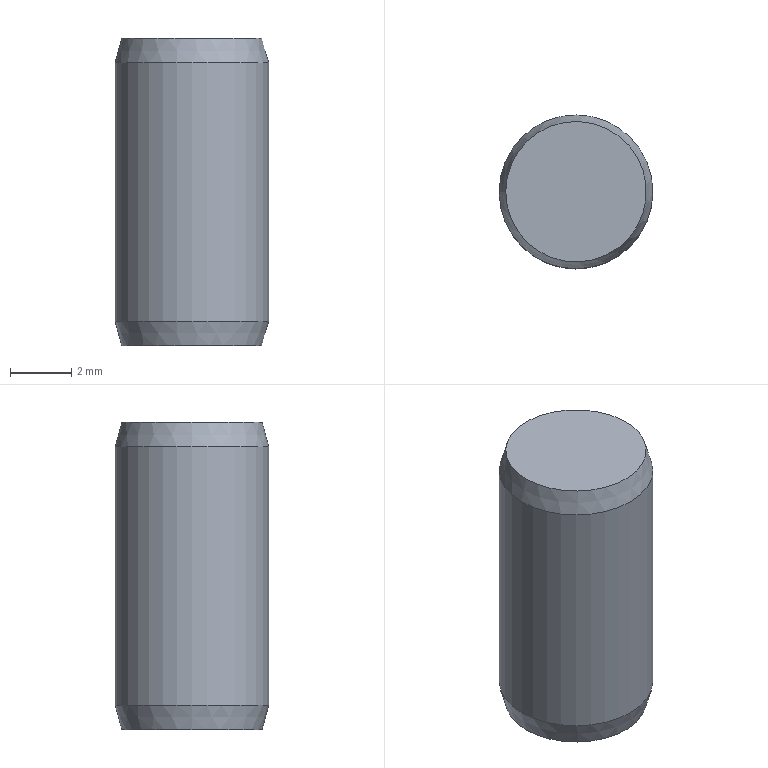Part | NX | features DATUM_CSYS 2, LINE 1, SKETCH 1, SWP104 1 | 1 solid | 5 faces | box 5 x 5 x 10 mm | volume 193.733 mm3 | plane 2 | cone 2 | cylinder 1 | commonest cylinder face diameters 5 x1
STEP:
#1=CARTESIAN_POINT('',(-2.286,0.,-10.));
#2=VERTEX_POINT('',#1);
#3=CARTESIAN_POINT('',(0.,0.,-10.));
#4=DIRECTION('',(0.,0.,-1.));
#5=DIRECTION('',(-1.,0.,0.));
#6=AXIS2_PLACEMENT_3D('',#3,#4,#5);
#7=CIRCLE('',#6,2.286);
#8=EDGE_CURVE('',#2,#2,#7,.T.);
#9=ORIENTED_EDGE('',*,*,#8,.T.);
#10=EDGE_LOOP('',(#9));
#11=FACE_BOUND('',#10,.T.);
#12=CARTESIAN_POINT('',(0.,0.,-10.));
#13=DIRECTION('',(0.,0.,-1.));
#14=DIRECTION('',(-1.,0.,0.));
#15=AXIS2_PLACEMENT_3D('',#12,#13,#14);
#16=PLANE('',#15);
#17=ADVANCED_FACE('',(#11),#16,.T.);
#18=CARTESIAN_POINT('',(-2.5,0.,-9.2));
#19=VERTEX_POINT('',#18);
#20=CARTESIAN_POINT('',(0.,0.,-9.2));
#21=DIRECTION('',(0.,0.,-1.));
#22=DIRECTION('',(-1.,0.,0.));
#23=AXIS2_PLACEMENT_3D('',#20,#21,#22);
#24=CIRCLE('',#23,2.5);
#25=EDGE_CURVE('',#19,#19,#24,.T.);
#26=ORIENTED_EDGE('',*,*,#25,.T.);
#27=EDGE_LOOP('',(#26));
#28=FACE_BOUND('',#27,.T.);
#29=ORIENTED_EDGE('',*,*,#8,.F.);
#30=EDGE_LOOP('',(#29));
#31=FACE_BOUND('',#30,.T.);
#32=CARTESIAN_POINT('',(0.,0.,-10.));
#33=DIRECTION('',(0.,0.,1.));
#34=DIRECTION('',(1.,0.,0.));
#35=AXIS2_PLACEMENT_3D('',#32,#33,#34);
#36=CONICAL_SURFACE('',#35,2.286,0.2618);
#37=ADVANCED_FACE('',(#28,#31),#36,.T.);
#38=CARTESIAN_POINT('',(-2.5,0.,-0.8));
#39=VERTEX_POINT('',#38);
#40=CARTESIAN_POINT('',(0.,0.,-0.8));
#41=DIRECTION('',(0.,0.,-1.));
#42=DIRECTION('',(-1.,0.,0.));
#43=AXIS2_PLACEMENT_3D('',#40,#41,#42);
#44=CIRCLE('',#43,2.5);
#45=EDGE_CURVE('',#39,#39,#44,.T.);
#46=ORIENTED_EDGE('',*,*,#45,.T.);
#47=EDGE_LOOP('',(#46));
#48=FACE_BOUND('',#47,.T.);
#49=ORIENTED_EDGE('',*,*,#25,.F.);
#50=EDGE_LOOP('',(#49));
#51=FACE_BOUND('',#50,.T.);
#52=CARTESIAN_POINT('',(0.,0.,0.));
#53=DIRECTION('',(0.,0.,-1.));
#54=DIRECTION('',(-1.,0.,0.));
#55=AXIS2_PLACEMENT_3D('',#52,#53,#54);
#56=CYLINDRICAL_SURFACE('',#55,2.5);
#57=ADVANCED_FACE('',(#48,#51),#56,.T.);
#58=CARTESIAN_POINT('',(-2.286,0.,0.));
#59=VERTEX_POINT('',#58);
#60=CARTESIAN_POINT('',(0.,0.,0.));
#61=DIRECTION('',(0.,0.,-1.));
#62=DIRECTION('',(-1.,0.,0.));
#63=AXIS2_PLACEMENT_3D('',#60,#61,#62);
#64=CIRCLE('',#63,2.286);
#65=EDGE_CURVE('',#59,#59,#64,.T.);
#66=ORIENTED_EDGE('',*,*,#65,.T.);
#67=EDGE_LOOP('',(#66));
#68=FACE_BOUND('',#67,.T.);
#69=ORIENTED_EDGE('',*,*,#45,.F.);
#70=EDGE_LOOP('',(#69));
#71=FACE_BOUND('',#70,.T.);
#72=CARTESIAN_POINT('',(0.,0.,-0.8));
#73=DIRECTION('',(0.,0.,-1.));
#74=DIRECTION('',(-1.,0.,0.));
#75=AXIS2_PLACEMENT_3D('',#72,#73,#74);
#76=CONICAL_SURFACE('',#75,2.5,0.2618);
#77=ADVANCED_FACE('',(#68,#71),#76,.T.);
#78=ORIENTED_EDGE('',*,*,#65,.F.);
#79=EDGE_LOOP('',(#78));
#80=FACE_BOUND('',#79,.T.);
#81=CARTESIAN_POINT('',(2.286,0.,0.));
#82=DIRECTION('',(0.,0.,1.));
#83=DIRECTION('',(1.,0.,0.));
#84=AXIS2_PLACEMENT_3D('',#81,#82,#83);
#85=PLANE('',#84);
#86=ADVANCED_FACE('',(#80),#85,.T.);
#87=CLOSED_SHELL('',(#17,#37,#57,#77,#86));
#88=MANIFOLD_SOLID_BREP('',#87);
#89=(LENGTH_UNIT()NAMED_UNIT(*)SI_UNIT(.MILLI.,.METRE.));
#90=UNCERTAINTY_MEASURE_WITH_UNIT(LENGTH_MEASURE(0.00001),#89,'','');
#91=(NAMED_UNIT(*)PLANE_ANGLE_UNIT()SI_UNIT($,.RADIAN.));
#92=(NAMED_UNIT(*)SI_UNIT($,.STERADIAN.)SOLID_ANGLE_UNIT());
#93=(GEOMETRIC_REPRESENTATION_CONTEXT(3)GLOBAL_UNCERTAINTY_ASSIGNED_CONTEXT((#90))GLOBAL_UNIT_ASSIGNED_CONTEXT((#89,#91,#92))REPRESENTATION_CONTEXT('',''));
#94=ADVANCED_BREP_SHAPE_REPRESENTATION('',(#88),#93);